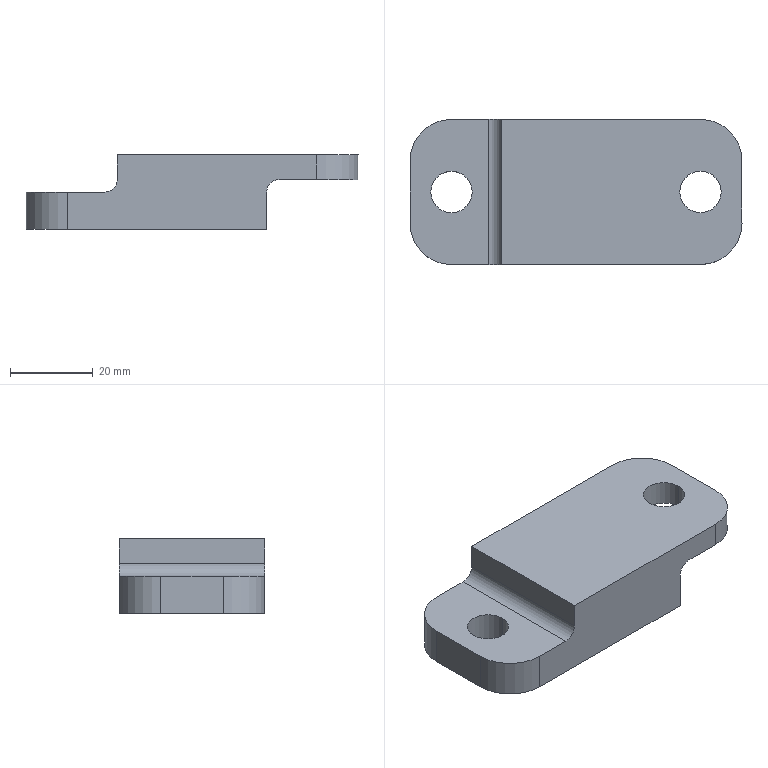Part | STEP file | Guard rod seat | 1 solid | 20 faces | box 80 x 35 x 18 mm | volume 32543 mm3 | cylinder 10 | plane 10 | commonest cylinder face diameters 10 x4 20 x4 6 x2